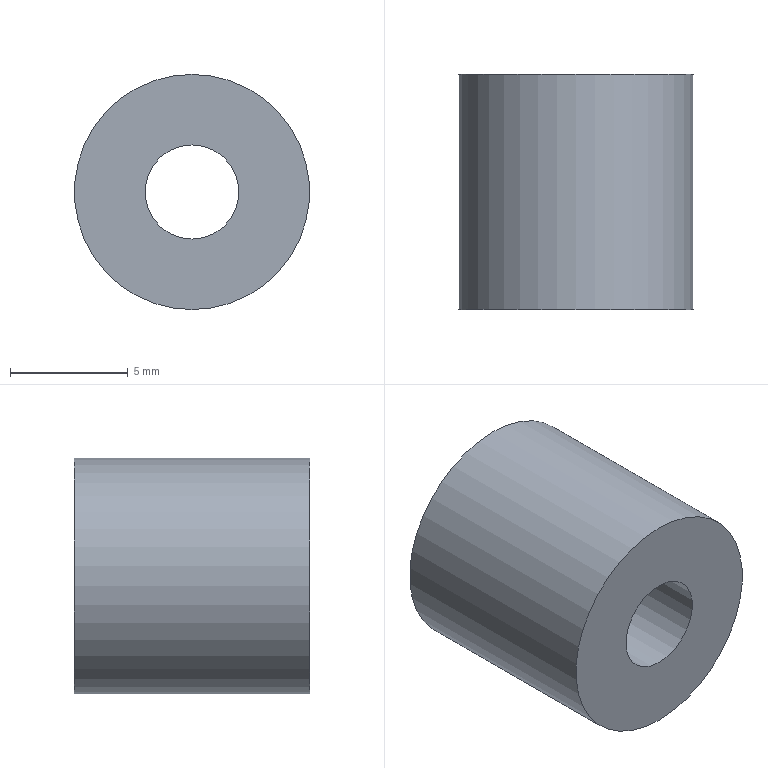Part | NX | features solid 2 | 1 solid | 4 faces | box 10 x 10 x 10 mm | volume 659.734 mm3 | cylinder 2 | plane 2 | commonest cylinder face diameters 4 x1 10 x1
STEP:
#1=CARTESIAN_POINT('',(-1160.,-410.,-56.));
#2=VERTEX_POINT('',#1);
#3=CARTESIAN_POINT('',(-1160.,-410.,-51.));
#4=DIRECTION('',(0.,1.,0.));
#5=DIRECTION('',(0.,0.,-1.));
#6=AXIS2_PLACEMENT_3D('',#3,#4,#5);
#7=CIRCLE('',#6,5.);
#8=EDGE_CURVE('',#2,#2,#7,.T.);
#9=ORIENTED_EDGE('',*,*,#8,.T.);
#10=EDGE_LOOP('',(#9));
#11=FACE_BOUND('',#10,.T.);
#12=CARTESIAN_POINT('',(-1160.,-400.,-56.));
#13=VERTEX_POINT('',#12);
#14=CARTESIAN_POINT('',(-1160.,-400.,-51.));
#15=DIRECTION('',(0.,1.,0.));
#16=DIRECTION('',(0.,0.,-1.));
#17=AXIS2_PLACEMENT_3D('',#14,#15,#16);
#18=CIRCLE('',#17,5.);
#19=EDGE_CURVE('',#13,#13,#18,.T.);
#20=ORIENTED_EDGE('',*,*,#19,.F.);
#21=EDGE_LOOP('',(#20));
#22=FACE_BOUND('',#21,.T.);
#23=CARTESIAN_POINT('',(-1160.,-410.,-51.));
#24=DIRECTION('',(0.,1.,0.));
#25=DIRECTION('',(0.,0.,-1.));
#26=AXIS2_PLACEMENT_3D('',#23,#24,#25);
#27=CYLINDRICAL_SURFACE('',#26,5.);
#28=ADVANCED_FACE('',(#11,#22),#27,.T.);
#29=CARTESIAN_POINT('',(-1160.,-410.,-53.));
#30=VERTEX_POINT('',#29);
#31=CARTESIAN_POINT('',(-1160.,-410.,-51.));
#32=DIRECTION('',(0.,1.,0.));
#33=DIRECTION('',(0.,0.,-1.));
#34=AXIS2_PLACEMENT_3D('',#31,#32,#33);
#35=CIRCLE('',#34,2.);
#36=EDGE_CURVE('',#30,#30,#35,.T.);
#37=ORIENTED_EDGE('',*,*,#36,.F.);
#38=EDGE_LOOP('',(#37));
#39=FACE_BOUND('',#38,.T.);
#40=CARTESIAN_POINT('',(-1160.,-400.,-53.));
#41=VERTEX_POINT('',#40);
#42=CARTESIAN_POINT('',(-1160.,-400.,-51.));
#43=DIRECTION('',(0.,1.,0.));
#44=DIRECTION('',(0.,0.,-1.));
#45=AXIS2_PLACEMENT_3D('',#42,#43,#44);
#46=CIRCLE('',#45,2.);
#47=EDGE_CURVE('',#41,#41,#46,.T.);
#48=ORIENTED_EDGE('',*,*,#47,.T.);
#49=EDGE_LOOP('',(#48));
#50=FACE_BOUND('',#49,.T.);
#51=CARTESIAN_POINT('',(-1160.,-410.,-51.));
#52=DIRECTION('',(0.,1.,0.));
#53=DIRECTION('',(0.,0.,-1.));
#54=AXIS2_PLACEMENT_3D('',#51,#52,#53);
#55=CYLINDRICAL_SURFACE('',#54,2.);
#56=ADVANCED_FACE('',(#39,#50),#55,.F.);
#57=ORIENTED_EDGE('',*,*,#8,.F.);
#58=EDGE_LOOP('',(#57));
#59=FACE_BOUND('',#58,.T.);
#60=ORIENTED_EDGE('',*,*,#36,.T.);
#61=EDGE_LOOP('',(#60));
#62=FACE_BOUND('',#61,.T.);
#63=CARTESIAN_POINT('',(-1160.,-410.,-51.));
#64=DIRECTION('',(0.,1.,0.));
#65=DIRECTION('',(0.,0.,-1.));
#66=AXIS2_PLACEMENT_3D('',#63,#64,#65);
#67=PLANE('',#66);
#68=ADVANCED_FACE('',(#59,#62),#67,.F.);
#69=ORIENTED_EDGE('',*,*,#19,.T.);
#70=EDGE_LOOP('',(#69));
#71=FACE_BOUND('',#70,.T.);
#72=ORIENTED_EDGE('',*,*,#47,.F.);
#73=EDGE_LOOP('',(#72));
#74=FACE_BOUND('',#73,.T.);
#75=CARTESIAN_POINT('',(-1160.,-400.,-51.));
#76=DIRECTION('',(0.,1.,0.));
#77=DIRECTION('',(0.,0.,-1.));
#78=AXIS2_PLACEMENT_3D('',#75,#76,#77);
#79=PLANE('',#78);
#80=ADVANCED_FACE('',(#71,#74),#79,.T.);
#81=CLOSED_SHELL('',(#28,#56,#68,#80));
#82=MANIFOLD_SOLID_BREP('',#81);
#83=(LENGTH_UNIT()NAMED_UNIT(*)SI_UNIT(.MILLI.,.METRE.));
#84=UNCERTAINTY_MEASURE_WITH_UNIT(LENGTH_MEASURE(0.00001),#83,'','');
#85=(NAMED_UNIT(*)PLANE_ANGLE_UNIT()SI_UNIT($,.RADIAN.));
#86=(NAMED_UNIT(*)SI_UNIT($,.STERADIAN.)SOLID_ANGLE_UNIT());
#87=(GEOMETRIC_REPRESENTATION_CONTEXT(3)GLOBAL_UNCERTAINTY_ASSIGNED_CONTEXT((#84))GLOBAL_UNIT_ASSIGNED_CONTEXT((#83,#85,#86))REPRESENTATION_CONTEXT('',''));
#88=ADVANCED_BREP_SHAPE_REPRESENTATION('',(#82),#87);